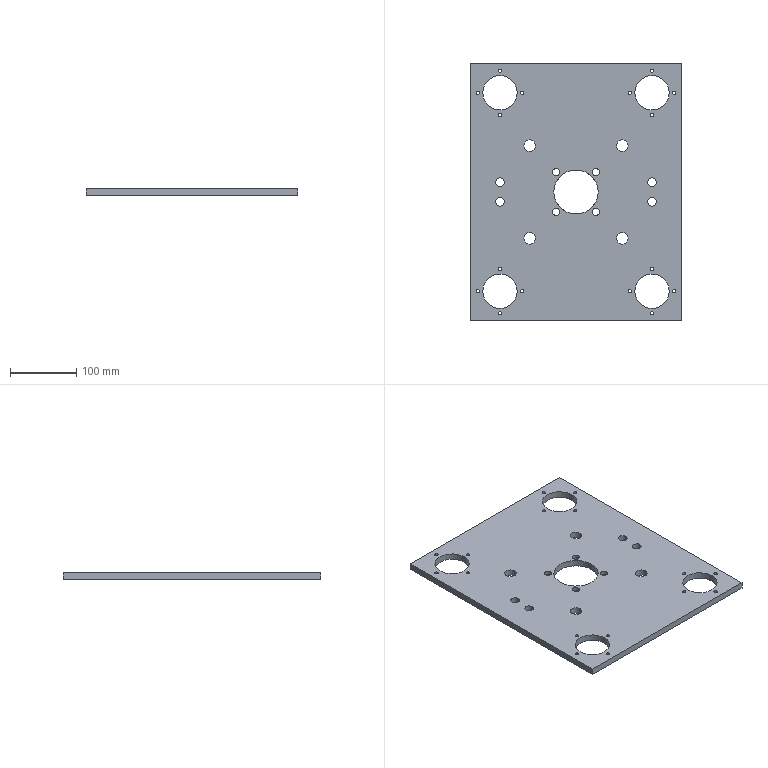Part | STEP file | 44-02-18 Locating Cylinder Mounting Plate | 1 solid | 80 faces | box 320 x 390 x 10 mm | volume 1104020 mm3 | cylinder 66 | cone 8 | plane 6 | commonest cylinder face diameters 5 x32 11 x8 13 x8 17.5 x8 52 x8 67 x2